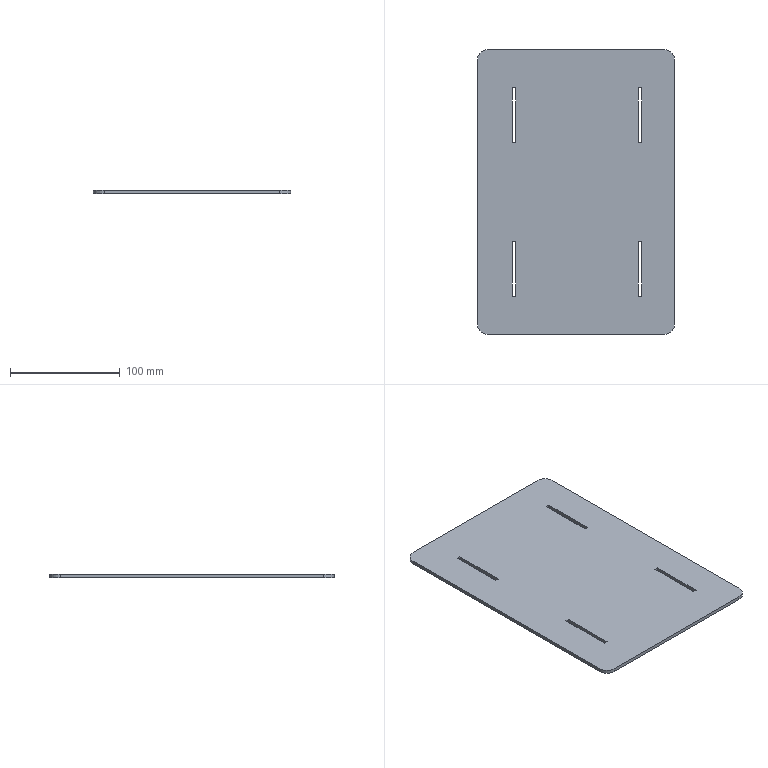Part | SolidWorks | features FlatPattern 1, SMBaseFlange 1, SheetMetal 1 | 1 solid | 26 faces | box 180 x 260 x 3.2 mm | volume 147437 mm3 | plane 22 | cylinder 4 | commonest cylinder face diameters 20 x4
STEP:
#1=CARTESIAN_POINT('',(-25.,119.865,3.2));
#2=VERTEX_POINT('',#1);
#3=CARTESIAN_POINT('',(-35.,109.865,3.2));
#4=VERTEX_POINT('',#3);
#5=CARTESIAN_POINT('',(-25.,109.865,3.2));
#6=DIRECTION('',(0.,0.,1.));
#7=DIRECTION('',(1.,0.,0.));
#8=AXIS2_PLACEMENT_3D('',#5,#6,#7);
#9=CIRCLE('',#8,10.);
#10=EDGE_CURVE('',#2,#4,#9,.T.);
#11=ORIENTED_EDGE('',*,*,#10,.T.);
#12=CARTESIAN_POINT('',(-35.,-130.135,3.2));
#13=VERTEX_POINT('',#12);
#14=CARTESIAN_POINT('',(-35.,109.865,3.2));
#15=DIRECTION('',(0.,-1.,0.));
#16=VECTOR('',#15,1000.);
#17=LINE('',#14,#16);
#18=EDGE_CURVE('',#4,#13,#17,.T.);
#19=ORIENTED_EDGE('',*,*,#18,.T.);
#20=CARTESIAN_POINT('',(-25.,-140.135,3.2));
#21=VERTEX_POINT('',#20);
#22=CARTESIAN_POINT('',(-25.,-130.135,3.2));
#23=DIRECTION('',(0.,0.,1.));
#24=DIRECTION('',(-1.,0.,0.));
#25=AXIS2_PLACEMENT_3D('',#22,#23,#24);
#26=CIRCLE('',#25,10.);
#27=EDGE_CURVE('',#13,#21,#26,.T.);
#28=ORIENTED_EDGE('',*,*,#27,.T.);
#29=CARTESIAN_POINT('',(135.,-140.135,3.2));
#30=VERTEX_POINT('',#29);
#31=CARTESIAN_POINT('',(135.,-140.135,3.2));
#32=DIRECTION('',(1.,0.,0.));
#33=VECTOR('',#32,1000.);
#34=LINE('',#31,#33);
#35=EDGE_CURVE('',#21,#30,#34,.T.);
#36=ORIENTED_EDGE('',*,*,#35,.T.);
#37=CARTESIAN_POINT('',(145.,-130.135,3.2));
#38=VERTEX_POINT('',#37);
#39=CARTESIAN_POINT('',(135.,-130.135,3.2));
#40=DIRECTION('',(0.,0.,1.));
#41=DIRECTION('',(-1.,0.,0.));
#42=AXIS2_PLACEMENT_3D('',#39,#40,#41);
#43=CIRCLE('',#42,10.);
#44=EDGE_CURVE('',#30,#38,#43,.T.);
#45=ORIENTED_EDGE('',*,*,#44,.T.);
#46=CARTESIAN_POINT('',(145.,109.865,3.2));
#47=VERTEX_POINT('',#46);
#48=CARTESIAN_POINT('',(145.,109.865,3.2));
#49=DIRECTION('',(0.,1.,0.));
#50=VECTOR('',#49,1000.);
#51=LINE('',#48,#50);
#52=EDGE_CURVE('',#38,#47,#51,.T.);
#53=ORIENTED_EDGE('',*,*,#52,.T.);
#54=CARTESIAN_POINT('',(135.,119.865,3.2));
#55=VERTEX_POINT('',#54);
#56=CARTESIAN_POINT('',(135.,109.865,3.2));
#57=DIRECTION('',(0.,0.,1.));
#58=DIRECTION('',(-1.,0.,0.));
#59=AXIS2_PLACEMENT_3D('',#56,#57,#58);
#60=CIRCLE('',#59,10.);
#61=EDGE_CURVE('',#47,#55,#60,.T.);
#62=ORIENTED_EDGE('',*,*,#61,.T.);
#63=CARTESIAN_POINT('',(135.,119.865,3.2));
#64=DIRECTION('',(-1.,0.,0.));
#65=VECTOR('',#64,1000.);
#66=LINE('',#63,#65);
#67=EDGE_CURVE('',#55,#2,#66,.T.);
#68=ORIENTED_EDGE('',*,*,#67,.T.);
#69=EDGE_LOOP('',(#11,#19,#28,#36,#45,#53,#62,#68));
#70=FACE_OUTER_BOUND('',#69,.T.);
#71=CARTESIAN_POINT('',(111.8,34.865,3.2));
#72=VERTEX_POINT('',#71);
#73=CARTESIAN_POINT('',(115.,34.865,3.2));
#74=VERTEX_POINT('',#73);
#75=CARTESIAN_POINT('',(111.8,34.865,3.2));
#76=DIRECTION('',(1.,0.,0.));
#77=VECTOR('',#76,1000.);
#78=LINE('',#75,#77);
#79=EDGE_CURVE('',#72,#74,#78,.T.);
#80=ORIENTED_EDGE('',*,*,#79,.F.);
#81=CARTESIAN_POINT('',(111.8,84.865,3.2));
#82=VERTEX_POINT('',#81);
#83=CARTESIAN_POINT('',(111.8,34.865,3.2));
#84=DIRECTION('',(0.,-1.,0.));
#85=VECTOR('',#84,1000.);
#86=LINE('',#83,#85);
#87=EDGE_CURVE('',#82,#72,#86,.T.);
#88=ORIENTED_EDGE('',*,*,#87,.F.);
#89=CARTESIAN_POINT('',(115.,84.865,3.2));
#90=VERTEX_POINT('',#89);
#91=CARTESIAN_POINT('',(111.8,84.865,3.2));
#92=DIRECTION('',(-1.,0.,0.));
#93=VECTOR('',#92,1000.);
#94=LINE('',#91,#93);
#95=EDGE_CURVE('',#90,#82,#94,.T.);
#96=ORIENTED_EDGE('',*,*,#95,.F.);
#97=CARTESIAN_POINT('',(115.,34.865,3.2));
#98=DIRECTION('',(0.,1.,0.));
#99=VECTOR('',#98,1000.);
#100=LINE('',#97,#99);
#101=EDGE_CURVE('',#74,#90,#100,.T.);
#102=ORIENTED_EDGE('',*,*,#101,.F.);
#103=EDGE_LOOP('',(#80,#88,#96,#102));
#104=FACE_BOUND('',#103,.T.);
#105=CARTESIAN_POINT('',(111.8,-105.135,3.2));
#106=VERTEX_POINT('',#105);
#107=CARTESIAN_POINT('',(115.,-105.135,3.2));
#108=VERTEX_POINT('',#107);
#109=CARTESIAN_POINT('',(111.8,-105.135,3.2));
#110=DIRECTION('',(1.,0.,0.));
#111=VECTOR('',#110,1000.);
#112=LINE('',#109,#111);
#113=EDGE_CURVE('',#106,#108,#112,.T.);
#114=ORIENTED_EDGE('',*,*,#113,.F.);
#115=CARTESIAN_POINT('',(111.8,-55.135,3.2));
#116=VERTEX_POINT('',#115);
#117=CARTESIAN_POINT('',(111.8,-55.135,3.2));
#118=DIRECTION('',(0.,-1.,0.));
#119=VECTOR('',#118,1000.);
#120=LINE('',#117,#119);
#121=EDGE_CURVE('',#116,#106,#120,.T.);
#122=ORIENTED_EDGE('',*,*,#121,.F.);
#123=CARTESIAN_POINT('',(115.,-55.135,3.2));
#124=VERTEX_POINT('',#123);
#125=CARTESIAN_POINT('',(111.8,-55.135,3.2));
#126=DIRECTION('',(-1.,0.,0.));
#127=VECTOR('',#126,1000.);
#128=LINE('',#125,#127);
#129=EDGE_CURVE('',#124,#116,#128,.T.);
#130=ORIENTED_EDGE('',*,*,#129,.F.);
#131=CARTESIAN_POINT('',(115.,-55.135,3.2));
#132=DIRECTION('',(0.,1.,0.));
#133=VECTOR('',#132,1000.);
#134=LINE('',#131,#133);
#135=EDGE_CURVE('',#108,#124,#134,.T.);
#136=ORIENTED_EDGE('',*,*,#135,.F.);
#137=EDGE_LOOP('',(#114,#122,#130,#136));
#138=FACE_BOUND('',#137,.T.);
#139=CARTESIAN_POINT('',(0.,-55.135,3.2));
#140=VERTEX_POINT('',#139);
#141=CARTESIAN_POINT('',(-3.2,-55.135,3.2));
#142=VERTEX_POINT('',#141);
#143=CARTESIAN_POINT('',(0.,-55.135,3.2));
#144=DIRECTION('',(-1.,0.,0.));
#145=VECTOR('',#144,1000.);
#146=LINE('',#143,#145);
#147=EDGE_CURVE('',#140,#142,#146,.T.);
#148=ORIENTED_EDGE('',*,*,#147,.F.);
#149=CARTESIAN_POINT('',(0.,-105.135,3.2));
#150=VERTEX_POINT('',#149);
#151=CARTESIAN_POINT('',(0.,-55.135,3.2));
#152=DIRECTION('',(0.,1.,0.));
#153=VECTOR('',#152,1000.);
#154=LINE('',#151,#153);
#155=EDGE_CURVE('',#150,#140,#154,.T.);
#156=ORIENTED_EDGE('',*,*,#155,.F.);
#157=CARTESIAN_POINT('',(-3.2,-105.135,3.2));
#158=VERTEX_POINT('',#157);
#159=CARTESIAN_POINT('',(0.,-105.135,3.2));
#160=DIRECTION('',(1.,0.,0.));
#161=VECTOR('',#160,1000.);
#162=LINE('',#159,#161);
#163=EDGE_CURVE('',#158,#150,#162,.T.);
#164=ORIENTED_EDGE('',*,*,#163,.F.);
#165=CARTESIAN_POINT('',(-3.2,-55.135,3.2));
#166=DIRECTION('',(0.,-1.,0.));
#167=VECTOR('',#166,1000.);
#168=LINE('',#165,#167);
#169=EDGE_CURVE('',#142,#158,#168,.T.);
#170=ORIENTED_EDGE('',*,*,#169,.F.);
#171=EDGE_LOOP('',(#148,#156,#164,#170));
#172=FACE_BOUND('',#171,.T.);
#173=CARTESIAN_POINT('',(0.,84.865,3.2));
#174=VERTEX_POINT('',#173);
#175=CARTESIAN_POINT('',(-3.2,84.865,3.2));
#176=VERTEX_POINT('',#175);
#177=CARTESIAN_POINT('',(0.,84.865,3.2));
#178=DIRECTION('',(-1.,0.,0.));
#179=VECTOR('',#178,1000.);
#180=LINE('',#177,#179);
#181=EDGE_CURVE('',#174,#176,#180,.T.);
#182=ORIENTED_EDGE('',*,*,#181,.F.);
#183=CARTESIAN_POINT('',(0.,34.865,3.2));
#184=VERTEX_POINT('',#183);
#185=CARTESIAN_POINT('',(0.,34.865,3.2));
#186=DIRECTION('',(0.,1.,0.));
#187=VECTOR('',#186,1000.);
#188=LINE('',#185,#187);
#189=EDGE_CURVE('',#184,#174,#188,.T.);
#190=ORIENTED_EDGE('',*,*,#189,.F.);
#191=CARTESIAN_POINT('',(-3.2,34.865,3.2));
#192=VERTEX_POINT('',#191);
#193=CARTESIAN_POINT('',(0.,34.865,3.2));
#194=DIRECTION('',(1.,0.,0.));
#195=VECTOR('',#194,1000.);
#196=LINE('',#193,#195);
#197=EDGE_CURVE('',#192,#184,#196,.T.);
#198=ORIENTED_EDGE('',*,*,#197,.F.);
#199=CARTESIAN_POINT('',(-3.2,34.865,3.2));
#200=DIRECTION('',(0.,-1.,0.));
#201=VECTOR('',#200,1000.);
#202=LINE('',#199,#201);
#203=EDGE_CURVE('',#176,#192,#202,.T.);
#204=ORIENTED_EDGE('',*,*,#203,.F.);
#205=EDGE_LOOP('',(#182,#190,#198,#204));
#206=FACE_BOUND('',#205,.T.);
#207=CARTESIAN_POINT('',(-25.,109.865,3.2));
#208=DIRECTION('',(0.,0.,1.));
#209=DIRECTION('',(1.,0.,0.));
#210=AXIS2_PLACEMENT_3D('',#207,#208,#209);
#211=PLANE('',#210);
#212=ADVANCED_FACE('',(#70,#104,#138,#172,#206),#211,.T.);
#213=CARTESIAN_POINT('',(0.,-105.135,0.));
#214=VERTEX_POINT('',#213);
#215=CARTESIAN_POINT('',(0.,-55.135,0.));
#216=VERTEX_POINT('',#215);
#217=CARTESIAN_POINT('',(0.,-55.135,0.));
#218=DIRECTION('',(0.,1.,0.));
#219=VECTOR('',#218,1000.);
#220=LINE('',#217,#219);
#221=EDGE_CURVE('',#214,#216,#220,.T.);
#222=ORIENTED_EDGE('',*,*,#221,.T.);
#223=CARTESIAN_POINT('',(-3.2,-55.135,0.));
#224=VERTEX_POINT('',#223);
#225=CARTESIAN_POINT('',(0.,-55.135,0.));
#226=DIRECTION('',(-1.,0.,0.));
#227=VECTOR('',#226,1000.);
#228=LINE('',#225,#227);
#229=EDGE_CURVE('',#216,#224,#228,.T.);
#230=ORIENTED_EDGE('',*,*,#229,.T.);
#231=CARTESIAN_POINT('',(-3.2,-105.135,0.));
#232=VERTEX_POINT('',#231);
#233=CARTESIAN_POINT('',(-3.2,-55.135,0.));
#234=DIRECTION('',(0.,-1.,0.));
#235=VECTOR('',#234,1000.);
#236=LINE('',#233,#235);
#237=EDGE_CURVE('',#224,#232,#236,.T.);
#238=ORIENTED_EDGE('',*,*,#237,.T.);
#239=CARTESIAN_POINT('',(0.,-105.135,0.));
#240=DIRECTION('',(1.,0.,0.));
#241=VECTOR('',#240,1000.);
#242=LINE('',#239,#241);
#243=EDGE_CURVE('',#232,#214,#242,.T.);
#244=ORIENTED_EDGE('',*,*,#243,.T.);
#245=EDGE_LOOP('',(#222,#230,#238,#244));
#246=FACE_BOUND('',#245,.T.);
#247=CARTESIAN_POINT('',(111.8,84.865,0.));
#248=VERTEX_POINT('',#247);
#249=CARTESIAN_POINT('',(111.8,34.865,0.));
#250=VERTEX_POINT('',#249);
#251=CARTESIAN_POINT('',(111.8,34.865,0.));
#252=DIRECTION('',(0.,-1.,0.));
#253=VECTOR('',#252,1000.);
#254=LINE('',#251,#253);
#255=EDGE_CURVE('',#248,#250,#254,.T.);
#256=ORIENTED_EDGE('',*,*,#255,.T.);
#257=CARTESIAN_POINT('',(115.,34.865,0.));
#258=VERTEX_POINT('',#257);
#259=CARTESIAN_POINT('',(111.8,34.865,0.));
#260=DIRECTION('',(1.,0.,0.));
#261=VECTOR('',#260,1000.);
#262=LINE('',#259,#261);
#263=EDGE_CURVE('',#250,#258,#262,.T.);
#264=ORIENTED_EDGE('',*,*,#263,.T.);
#265=CARTESIAN_POINT('',(115.,84.865,0.));
#266=VERTEX_POINT('',#265);
#267=CARTESIAN_POINT('',(115.,34.865,0.));
#268=DIRECTION('',(0.,1.,0.));
#269=VECTOR('',#268,1000.);
#270=LINE('',#267,#269);
#271=EDGE_CURVE('',#258,#266,#270,.T.);
#272=ORIENTED_EDGE('',*,*,#271,.T.);
#273=CARTESIAN_POINT('',(111.8,84.865,0.));
#274=DIRECTION('',(-1.,0.,0.));
#275=VECTOR('',#274,1000.);
#276=LINE('',#273,#275);
#277=EDGE_CURVE('',#266,#248,#276,.T.);
#278=ORIENTED_EDGE('',*,*,#277,.T.);
#279=EDGE_LOOP('',(#256,#264,#272,#278));
#280=FACE_BOUND('',#279,.T.);
#281=CARTESIAN_POINT('',(-25.,119.865,0.));
#282=VERTEX_POINT('',#281);
#283=CARTESIAN_POINT('',(-35.,109.865,0.));
#284=VERTEX_POINT('',#283);
#285=CARTESIAN_POINT('',(-25.,109.865,0.));
#286=DIRECTION('',(0.,0.,1.));
#287=DIRECTION('',(1.,0.,0.));
#288=AXIS2_PLACEMENT_3D('',#285,#286,#287);
#289=CIRCLE('',#288,10.);
#290=EDGE_CURVE('',#282,#284,#289,.T.);
#291=ORIENTED_EDGE('',*,*,#290,.F.);
#292=CARTESIAN_POINT('',(135.,119.865,0.));
#293=VERTEX_POINT('',#292);
#294=CARTESIAN_POINT('',(135.,119.865,0.));
#295=DIRECTION('',(-1.,0.,0.));
#296=VECTOR('',#295,1000.);
#297=LINE('',#294,#296);
#298=EDGE_CURVE('',#293,#282,#297,.T.);
#299=ORIENTED_EDGE('',*,*,#298,.F.);
#300=CARTESIAN_POINT('',(145.,109.865,0.));
#301=VERTEX_POINT('',#300);
#302=CARTESIAN_POINT('',(135.,109.865,0.));
#303=DIRECTION('',(0.,0.,1.));
#304=DIRECTION('',(-1.,0.,0.));
#305=AXIS2_PLACEMENT_3D('',#302,#303,#304);
#306=CIRCLE('',#305,10.);
#307=EDGE_CURVE('',#301,#293,#306,.T.);
#308=ORIENTED_EDGE('',*,*,#307,.F.);
#309=CARTESIAN_POINT('',(145.,-130.135,0.));
#310=VERTEX_POINT('',#309);
#311=CARTESIAN_POINT('',(145.,109.865,0.));
#312=DIRECTION('',(0.,1.,0.));
#313=VECTOR('',#312,1000.);
#314=LINE('',#311,#313);
#315=EDGE_CURVE('',#310,#301,#314,.T.);
#316=ORIENTED_EDGE('',*,*,#315,.F.);
#317=CARTESIAN_POINT('',(135.,-140.135,0.));
#318=VERTEX_POINT('',#317);
#319=CARTESIAN_POINT('',(135.,-130.135,0.));
#320=DIRECTION('',(0.,0.,1.));
#321=DIRECTION('',(-1.,0.,0.));
#322=AXIS2_PLACEMENT_3D('',#319,#320,#321);
#323=CIRCLE('',#322,10.);
#324=EDGE_CURVE('',#318,#310,#323,.T.);
#325=ORIENTED_EDGE('',*,*,#324,.F.);
#326=CARTESIAN_POINT('',(-25.,-140.135,0.));
#327=VERTEX_POINT('',#326);
#328=CARTESIAN_POINT('',(135.,-140.135,0.));
#329=DIRECTION('',(1.,0.,0.));
#330=VECTOR('',#329,1000.);
#331=LINE('',#328,#330);
#332=EDGE_CURVE('',#327,#318,#331,.T.);
#333=ORIENTED_EDGE('',*,*,#332,.F.);
#334=CARTESIAN_POINT('',(-35.,-130.135,0.));
#335=VERTEX_POINT('',#334);
#336=CARTESIAN_POINT('',(-25.,-130.135,0.));
#337=DIRECTION('',(0.,0.,1.));
#338=DIRECTION('',(-1.,0.,0.));
#339=AXIS2_PLACEMENT_3D('',#336,#337,#338);
#340=CIRCLE('',#339,10.);
#341=EDGE_CURVE('',#335,#327,#340,.T.);
#342=ORIENTED_EDGE('',*,*,#341,.F.);
#343=CARTESIAN_POINT('',(-35.,109.865,0.));
#344=DIRECTION('',(0.,-1.,0.));
#345=VECTOR('',#344,1000.);
#346=LINE('',#343,#345);
#347=EDGE_CURVE('',#284,#335,#346,.T.);
#348=ORIENTED_EDGE('',*,*,#347,.F.);
#349=EDGE_LOOP('',(#291,#299,#308,#316,#325,#333,#342,#348));
#350=FACE_OUTER_BOUND('',#349,.T.);
#351=CARTESIAN_POINT('',(111.8,-55.135,0.));
#352=VERTEX_POINT('',#351);
#353=CARTESIAN_POINT('',(111.8,-105.135,0.));
#354=VERTEX_POINT('',#353);
#355=CARTESIAN_POINT('',(111.8,-55.135,0.));
#356=DIRECTION('',(0.,-1.,0.));
#357=VECTOR('',#356,1000.);
#358=LINE('',#355,#357);
#359=EDGE_CURVE('',#352,#354,#358,.T.);
#360=ORIENTED_EDGE('',*,*,#359,.T.);
#361=CARTESIAN_POINT('',(115.,-105.135,0.));
#362=VERTEX_POINT('',#361);
#363=CARTESIAN_POINT('',(111.8,-105.135,0.));
#364=DIRECTION('',(1.,0.,0.));
#365=VECTOR('',#364,1000.);
#366=LINE('',#363,#365);
#367=EDGE_CURVE('',#354,#362,#366,.T.);
#368=ORIENTED_EDGE('',*,*,#367,.T.);
#369=CARTESIAN_POINT('',(115.,-55.135,0.));
#370=VERTEX_POINT('',#369);
#371=CARTESIAN_POINT('',(115.,-55.135,0.));
#372=DIRECTION('',(0.,1.,0.));
#373=VECTOR('',#372,1000.);
#374=LINE('',#371,#373);
#375=EDGE_CURVE('',#362,#370,#374,.T.);
#376=ORIENTED_EDGE('',*,*,#375,.T.);
#377=CARTESIAN_POINT('',(111.8,-55.135,0.));
#378=DIRECTION('',(-1.,0.,0.));
#379=VECTOR('',#378,1000.);
#380=LINE('',#377,#379);
#381=EDGE_CURVE('',#370,#352,#380,.T.);
#382=ORIENTED_EDGE('',*,*,#381,.T.);
#383=EDGE_LOOP('',(#360,#368,#376,#382));
#384=FACE_BOUND('',#383,.T.);
#385=CARTESIAN_POINT('',(0.,34.865,0.));
#386=VERTEX_POINT('',#385);
#387=CARTESIAN_POINT('',(0.,84.865,0.));
#388=VERTEX_POINT('',#387);
#389=CARTESIAN_POINT('',(0.,34.865,0.));
#390=DIRECTION('',(0.,1.,0.));
#391=VECTOR('',#390,1000.);
#392=LINE('',#389,#391);
#393=EDGE_CURVE('',#386,#388,#392,.T.);
#394=ORIENTED_EDGE('',*,*,#393,.T.);
#395=CARTESIAN_POINT('',(-3.2,84.865,0.));
#396=VERTEX_POINT('',#395);
#397=CARTESIAN_POINT('',(0.,84.865,0.));
#398=DIRECTION('',(-1.,0.,0.));
#399=VECTOR('',#398,1000.);
#400=LINE('',#397,#399);
#401=EDGE_CURVE('',#388,#396,#400,.T.);
#402=ORIENTED_EDGE('',*,*,#401,.T.);
#403=CARTESIAN_POINT('',(-3.2,34.865,0.));
#404=VERTEX_POINT('',#403);
#405=CARTESIAN_POINT('',(-3.2,34.865,0.));
#406=DIRECTION('',(0.,-1.,0.));
#407=VECTOR('',#406,1000.);
#408=LINE('',#405,#407);
#409=EDGE_CURVE('',#396,#404,#408,.T.);
#410=ORIENTED_EDGE('',*,*,#409,.T.);
#411=CARTESIAN_POINT('',(0.,34.865,0.));
#412=DIRECTION('',(1.,0.,0.));
#413=VECTOR('',#412,1000.);
#414=LINE('',#411,#413);
#415=EDGE_CURVE('',#404,#386,#414,.T.);
#416=ORIENTED_EDGE('',*,*,#415,.T.);
#417=EDGE_LOOP('',(#394,#402,#410,#416));
#418=FACE_BOUND('',#417,.T.);
#419=CARTESIAN_POINT('',(-25.,109.865,0.));
#420=DIRECTION('',(0.,0.,1.));
#421=DIRECTION('',(1.,0.,0.));
#422=AXIS2_PLACEMENT_3D('',#419,#420,#421);
#423=PLANE('',#422);
#424=ADVANCED_FACE('',(#246,#280,#350,#384,#418),#423,.F.);
#425=ORIENTED_EDGE('',*,*,#290,.T.);
#426=CARTESIAN_POINT('',(-35.,109.865,3.2));
#427=DIRECTION('',(0.,0.,-1.));
#428=VECTOR('',#427,1000.);
#429=LINE('',#426,#428);
#430=EDGE_CURVE('',#4,#284,#429,.T.);
#431=ORIENTED_EDGE('',*,*,#430,.F.);
#432=ORIENTED_EDGE('',*,*,#10,.F.);
#433=CARTESIAN_POINT('',(-25.,119.865,3.2));
#434=DIRECTION('',(0.,0.,-1.));
#435=VECTOR('',#434,1000.);
#436=LINE('',#433,#435);
#437=EDGE_CURVE('',#2,#282,#436,.T.);
#438=ORIENTED_EDGE('',*,*,#437,.T.);
#439=EDGE_LOOP('',(#425,#431,#432,#438));
#440=FACE_OUTER_BOUND('',#439,.T.);
#441=CARTESIAN_POINT('',(-25.,109.865,3.2));
#442=DIRECTION('',(0.,0.,-1.));
#443=DIRECTION('',(-1.,0.,0.));
#444=AXIS2_PLACEMENT_3D('',#441,#442,#443);
#445=CYLINDRICAL_SURFACE('',#444,10.);
#446=ADVANCED_FACE('',(#440),#445,.T.);
#447=ORIENTED_EDGE('',*,*,#347,.T.);
#448=CARTESIAN_POINT('',(-35.,-130.135,3.2));
#449=DIRECTION('',(0.,0.,-1.));
#450=VECTOR('',#449,1000.);
#451=LINE('',#448,#450);
#452=EDGE_CURVE('',#13,#335,#451,.T.);
#453=ORIENTED_EDGE('',*,*,#452,.F.);
#454=ORIENTED_EDGE('',*,*,#18,.F.);
#455=ORIENTED_EDGE('',*,*,#430,.T.);
#456=EDGE_LOOP('',(#447,#453,#454,#455));
#457=FACE_OUTER_BOUND('',#456,.T.);
#458=CARTESIAN_POINT('',(-35.,109.865,3.2));
#459=DIRECTION('',(1.,0.,0.));
#460=DIRECTION('',(0.,1.,0.));
#461=AXIS2_PLACEMENT_3D('',#458,#459,#460);
#462=PLANE('',#461);
#463=ADVANCED_FACE('',(#457),#462,.F.);
#464=ORIENTED_EDGE('',*,*,#341,.T.);
#465=CARTESIAN_POINT('',(-25.,-140.135,3.2));
#466=DIRECTION('',(0.,0.,-1.));
#467=VECTOR('',#466,1000.);
#468=LINE('',#465,#467);
#469=EDGE_CURVE('',#21,#327,#468,.T.);
#470=ORIENTED_EDGE('',*,*,#469,.F.);
#471=ORIENTED_EDGE('',*,*,#27,.F.);
#472=ORIENTED_EDGE('',*,*,#452,.T.);
#473=EDGE_LOOP('',(#464,#470,#471,#472));
#474=FACE_OUTER_BOUND('',#473,.T.);
#475=CARTESIAN_POINT('',(-25.,-130.135,3.2));
#476=DIRECTION('',(0.,0.,-1.));
#477=DIRECTION('',(-1.,0.,0.));
#478=AXIS2_PLACEMENT_3D('',#475,#476,#477);
#479=CYLINDRICAL_SURFACE('',#478,10.);
#480=ADVANCED_FACE('',(#474),#479,.T.);
#481=ORIENTED_EDGE('',*,*,#332,.T.);
#482=CARTESIAN_POINT('',(135.,-140.135,3.2));
#483=DIRECTION('',(0.,0.,-1.));
#484=VECTOR('',#483,1000.);
#485=LINE('',#482,#484);
#486=EDGE_CURVE('',#30,#318,#485,.T.);
#487=ORIENTED_EDGE('',*,*,#486,.F.);
#488=ORIENTED_EDGE('',*,*,#35,.F.);
#489=ORIENTED_EDGE('',*,*,#469,.T.);
#490=EDGE_LOOP('',(#481,#487,#488,#489));
#491=FACE_OUTER_BOUND('',#490,.T.);
#492=CARTESIAN_POINT('',(135.,-140.135,3.2));
#493=DIRECTION('',(0.,1.,0.));
#494=DIRECTION('',(0.,0.,1.));
#495=AXIS2_PLACEMENT_3D('',#492,#493,#494);
#496=PLANE('',#495);
#497=ADVANCED_FACE('',(#491),#496,.F.);
#498=ORIENTED_EDGE('',*,*,#324,.T.);
#499=CARTESIAN_POINT('',(145.,-130.135,3.2));
#500=DIRECTION('',(0.,0.,-1.));
#501=VECTOR('',#500,1000.);
#502=LINE('',#499,#501);
#503=EDGE_CURVE('',#38,#310,#502,.T.);
#504=ORIENTED_EDGE('',*,*,#503,.F.);
#505=ORIENTED_EDGE('',*,*,#44,.F.);
#506=ORIENTED_EDGE('',*,*,#486,.T.);
#507=EDGE_LOOP('',(#498,#504,#505,#506));
#508=FACE_OUTER_BOUND('',#507,.T.);
#509=CARTESIAN_POINT('',(135.,-130.135,3.2));
#510=DIRECTION('',(0.,0.,-1.));
#511=DIRECTION('',(-1.,0.,0.));
#512=AXIS2_PLACEMENT_3D('',#509,#510,#511);
#513=CYLINDRICAL_SURFACE('',#512,10.);
#514=ADVANCED_FACE('',(#508),#513,.T.);
#515=ORIENTED_EDGE('',*,*,#315,.T.);
#516=CARTESIAN_POINT('',(145.,109.865,3.2));
#517=DIRECTION('',(0.,0.,-1.));
#518=VECTOR('',#517,1000.);
#519=LINE('',#516,#518);
#520=EDGE_CURVE('',#47,#301,#519,.T.);
#521=ORIENTED_EDGE('',*,*,#520,.F.);
#522=ORIENTED_EDGE('',*,*,#52,.F.);
#523=ORIENTED_EDGE('',*,*,#503,.T.);
#524=EDGE_LOOP('',(#515,#521,#522,#523));
#525=FACE_OUTER_BOUND('',#524,.T.);
#526=CARTESIAN_POINT('',(145.,109.865,3.2));
#527=DIRECTION('',(-1.,0.,0.));
#528=DIRECTION('',(0.,-1.,0.));
#529=AXIS2_PLACEMENT_3D('',#526,#527,#528);
#530=PLANE('',#529);
#531=ADVANCED_FACE('',(#525),#530,.F.);
#532=ORIENTED_EDGE('',*,*,#307,.T.);
#533=CARTESIAN_POINT('',(135.,119.865,3.2));
#534=DIRECTION('',(0.,0.,-1.));
#535=VECTOR('',#534,1000.);
#536=LINE('',#533,#535);
#537=EDGE_CURVE('',#55,#293,#536,.T.);
#538=ORIENTED_EDGE('',*,*,#537,.F.);
#539=ORIENTED_EDGE('',*,*,#61,.F.);
#540=ORIENTED_EDGE('',*,*,#520,.T.);
#541=EDGE_LOOP('',(#532,#538,#539,#540));
#542=FACE_OUTER_BOUND('',#541,.T.);
#543=CARTESIAN_POINT('',(135.,109.865,3.2));
#544=DIRECTION('',(0.,0.,-1.));
#545=DIRECTION('',(-1.,0.,0.));
#546=AXIS2_PLACEMENT_3D('',#543,#544,#545);
#547=CYLINDRICAL_SURFACE('',#546,10.);
#548=ADVANCED_FACE('',(#542),#547,.T.);
#549=ORIENTED_EDGE('',*,*,#298,.T.);
#550=ORIENTED_EDGE('',*,*,#437,.F.);
#551=ORIENTED_EDGE('',*,*,#67,.F.);
#552=ORIENTED_EDGE('',*,*,#537,.T.);
#553=EDGE_LOOP('',(#549,#550,#551,#552));
#554=FACE_OUTER_BOUND('',#553,.T.);
#555=CARTESIAN_POINT('',(135.,119.865,3.2));
#556=DIRECTION('',(0.,-1.,0.));
#557=DIRECTION('',(1.,0.,0.));
#558=AXIS2_PLACEMENT_3D('',#555,#556,#557);
#559=PLANE('',#558);
#560=ADVANCED_FACE('',(#554),#559,.F.);
#561=ORIENTED_EDGE('',*,*,#255,.F.);
#562=CARTESIAN_POINT('',(111.8,84.865,3.2));
#563=DIRECTION('',(0.,0.,-1.));
#564=VECTOR('',#563,1000.);
#565=LINE('',#562,#564);
#566=EDGE_CURVE('',#82,#248,#565,.T.);
#567=ORIENTED_EDGE('',*,*,#566,.F.);
#568=ORIENTED_EDGE('',*,*,#87,.T.);
#569=CARTESIAN_POINT('',(111.8,34.865,3.2));
#570=DIRECTION('',(0.,0.,-1.));
#571=VECTOR('',#570,1000.);
#572=LINE('',#569,#571);
#573=EDGE_CURVE('',#72,#250,#572,.T.);
#574=ORIENTED_EDGE('',*,*,#573,.T.);
#575=EDGE_LOOP('',(#561,#567,#568,#574));
#576=FACE_OUTER_BOUND('',#575,.T.);
#577=CARTESIAN_POINT('',(111.8,34.865,3.2));
#578=DIRECTION('',(1.,0.,0.));
#579=DIRECTION('',(0.,0.,-1.));
#580=AXIS2_PLACEMENT_3D('',#577,#578,#579);
#581=PLANE('',#580);
#582=ADVANCED_FACE('',(#576),#581,.T.);
#583=ORIENTED_EDGE('',*,*,#263,.F.);
#584=ORIENTED_EDGE('',*,*,#573,.F.);
#585=ORIENTED_EDGE('',*,*,#79,.T.);
#586=CARTESIAN_POINT('',(115.,34.865,3.2));
#587=DIRECTION('',(0.,0.,-1.));
#588=VECTOR('',#587,1000.);
#589=LINE('',#586,#588);
#590=EDGE_CURVE('',#74,#258,#589,.T.);
#591=ORIENTED_EDGE('',*,*,#590,.T.);
#592=EDGE_LOOP('',(#583,#584,#585,#591));
#593=FACE_OUTER_BOUND('',#592,.T.);
#594=CARTESIAN_POINT('',(111.8,34.865,3.2));
#595=DIRECTION('',(0.,1.,0.));
#596=DIRECTION('',(0.,0.,1.));
#597=AXIS2_PLACEMENT_3D('',#594,#595,#596);
#598=PLANE('',#597);
#599=ADVANCED_FACE('',(#593),#598,.T.);
#600=ORIENTED_EDGE('',*,*,#271,.F.);
#601=ORIENTED_EDGE('',*,*,#590,.F.);
#602=ORIENTED_EDGE('',*,*,#101,.T.);
#603=CARTESIAN_POINT('',(115.,84.865,3.2));
#604=DIRECTION('',(0.,0.,-1.));
#605=VECTOR('',#604,1000.);
#606=LINE('',#603,#605);
#607=EDGE_CURVE('',#90,#266,#606,.T.);
#608=ORIENTED_EDGE('',*,*,#607,.T.);
#609=EDGE_LOOP('',(#600,#601,#602,#608));
#610=FACE_OUTER_BOUND('',#609,.T.);
#611=CARTESIAN_POINT('',(115.,34.865,3.2));
#612=DIRECTION('',(-1.,0.,0.));
#613=DIRECTION('',(0.,0.,1.));
#614=AXIS2_PLACEMENT_3D('',#611,#612,#613);
#615=PLANE('',#614);
#616=ADVANCED_FACE('',(#610),#615,.T.);
#617=ORIENTED_EDGE('',*,*,#277,.F.);
#618=ORIENTED_EDGE('',*,*,#607,.F.);
#619=ORIENTED_EDGE('',*,*,#95,.T.);
#620=ORIENTED_EDGE('',*,*,#566,.T.);
#621=EDGE_LOOP('',(#617,#618,#619,#620));
#622=FACE_OUTER_BOUND('',#621,.T.);
#623=CARTESIAN_POINT('',(111.8,84.865,3.2));
#624=DIRECTION('',(0.,-1.,0.));
#625=DIRECTION('',(0.,0.,-1.));
#626=AXIS2_PLACEMENT_3D('',#623,#624,#625);
#627=PLANE('',#626);
#628=ADVANCED_FACE('',(#622),#627,.T.);
#629=ORIENTED_EDGE('',*,*,#359,.F.);
#630=CARTESIAN_POINT('',(111.8,-55.135,3.2));
#631=DIRECTION('',(0.,0.,-1.));
#632=VECTOR('',#631,1000.);
#633=LINE('',#630,#632);
#634=EDGE_CURVE('',#116,#352,#633,.T.);
#635=ORIENTED_EDGE('',*,*,#634,.F.);
#636=ORIENTED_EDGE('',*,*,#121,.T.);
#637=CARTESIAN_POINT('',(111.8,-105.135,3.2));
#638=DIRECTION('',(0.,0.,-1.));
#639=VECTOR('',#638,1000.);
#640=LINE('',#637,#639);
#641=EDGE_CURVE('',#106,#354,#640,.T.);
#642=ORIENTED_EDGE('',*,*,#641,.T.);
#643=EDGE_LOOP('',(#629,#635,#636,#642));
#644=FACE_OUTER_BOUND('',#643,.T.);
#645=CARTESIAN_POINT('',(111.8,-55.135,3.2));
#646=DIRECTION('',(1.,0.,0.));
#647=DIRECTION('',(0.,0.,-1.));
#648=AXIS2_PLACEMENT_3D('',#645,#646,#647);
#649=PLANE('',#648);
#650=ADVANCED_FACE('',(#644),#649,.T.);
#651=ORIENTED_EDGE('',*,*,#367,.F.);
#652=ORIENTED_EDGE('',*,*,#641,.F.);
#653=ORIENTED_EDGE('',*,*,#113,.T.);
#654=CARTESIAN_POINT('',(115.,-105.135,3.2));
#655=DIRECTION('',(0.,0.,-1.));
#656=VECTOR('',#655,1000.);
#657=LINE('',#654,#656);
#658=EDGE_CURVE('',#108,#362,#657,.T.);
#659=ORIENTED_EDGE('',*,*,#658,.T.);
#660=EDGE_LOOP('',(#651,#652,#653,#659));
#661=FACE_OUTER_BOUND('',#660,.T.);
#662=CARTESIAN_POINT('',(111.8,-105.135,3.2));
#663=DIRECTION('',(0.,1.,0.));
#664=DIRECTION('',(0.,0.,1.));
#665=AXIS2_PLACEMENT_3D('',#662,#663,#664);
#666=PLANE('',#665);
#667=ADVANCED_FACE('',(#661),#666,.T.);
#668=ORIENTED_EDGE('',*,*,#375,.F.);
#669=ORIENTED_EDGE('',*,*,#658,.F.);
#670=ORIENTED_EDGE('',*,*,#135,.T.);
#671=CARTESIAN_POINT('',(115.,-55.135,3.2));
#672=DIRECTION('',(0.,0.,-1.));
#673=VECTOR('',#672,1000.);
#674=LINE('',#671,#673);
#675=EDGE_CURVE('',#124,#370,#674,.T.);
#676=ORIENTED_EDGE('',*,*,#675,.T.);
#677=EDGE_LOOP('',(#668,#669,#670,#676));
#678=FACE_OUTER_BOUND('',#677,.T.);
#679=CARTESIAN_POINT('',(115.,-55.135,3.2));
#680=DIRECTION('',(-1.,0.,0.));
#681=DIRECTION('',(0.,0.,1.));
#682=AXIS2_PLACEMENT_3D('',#679,#680,#681);
#683=PLANE('',#682);
#684=ADVANCED_FACE('',(#678),#683,.T.);
#685=ORIENTED_EDGE('',*,*,#381,.F.);
#686=ORIENTED_EDGE('',*,*,#675,.F.);
#687=ORIENTED_EDGE('',*,*,#129,.T.);
#688=ORIENTED_EDGE('',*,*,#634,.T.);
#689=EDGE_LOOP('',(#685,#686,#687,#688));
#690=FACE_OUTER_BOUND('',#689,.T.);
#691=CARTESIAN_POINT('',(111.8,-55.135,3.2));
#692=DIRECTION('',(0.,-1.,0.));
#693=DIRECTION('',(0.,0.,-1.));
#694=AXIS2_PLACEMENT_3D('',#691,#692,#693);
#695=PLANE('',#694);
#696=ADVANCED_FACE('',(#690),#695,.T.);
#697=ORIENTED_EDGE('',*,*,#221,.F.);
#698=CARTESIAN_POINT('',(0.,-105.135,3.2));
#699=DIRECTION('',(0.,0.,-1.));
#700=VECTOR('',#699,1000.);
#701=LINE('',#698,#700);
#702=EDGE_CURVE('',#150,#214,#701,.T.);
#703=ORIENTED_EDGE('',*,*,#702,.F.);
#704=ORIENTED_EDGE('',*,*,#155,.T.);
#705=CARTESIAN_POINT('',(0.,-55.135,3.2));
#706=DIRECTION('',(0.,0.,-1.));
#707=VECTOR('',#706,1000.);
#708=LINE('',#705,#707);
#709=EDGE_CURVE('',#140,#216,#708,.T.);
#710=ORIENTED_EDGE('',*,*,#709,.T.);
#711=EDGE_LOOP('',(#697,#703,#704,#710));
#712=FACE_OUTER_BOUND('',#711,.T.);
#713=CARTESIAN_POINT('',(0.,-55.135,3.2));
#714=DIRECTION('',(-1.,0.,0.));
#715=DIRECTION('',(0.,0.,1.));
#716=AXIS2_PLACEMENT_3D('',#713,#714,#715);
#717=PLANE('',#716);
#718=ADVANCED_FACE('',(#712),#717,.T.);
#719=ORIENTED_EDGE('',*,*,#229,.F.);
#720=ORIENTED_EDGE('',*,*,#709,.F.);
#721=ORIENTED_EDGE('',*,*,#147,.T.);
#722=CARTESIAN_POINT('',(-3.2,-55.135,3.2));
#723=DIRECTION('',(0.,0.,-1.));
#724=VECTOR('',#723,1000.);
#725=LINE('',#722,#724);
#726=EDGE_CURVE('',#142,#224,#725,.T.);
#727=ORIENTED_EDGE('',*,*,#726,.T.);
#728=EDGE_LOOP('',(#719,#720,#721,#727));
#729=FACE_OUTER_BOUND('',#728,.T.);
#730=CARTESIAN_POINT('',(0.,-55.135,3.2));
#731=DIRECTION('',(0.,-1.,0.));
#732=DIRECTION('',(0.,0.,-1.));
#733=AXIS2_PLACEMENT_3D('',#730,#731,#732);
#734=PLANE('',#733);
#735=ADVANCED_FACE('',(#729),#734,.T.);
#736=ORIENTED_EDGE('',*,*,#237,.F.);
#737=ORIENTED_EDGE('',*,*,#726,.F.);
#738=ORIENTED_EDGE('',*,*,#169,.T.);
#739=CARTESIAN_POINT('',(-3.2,-105.135,3.2));
#740=DIRECTION('',(0.,0.,-1.));
#741=VECTOR('',#740,1000.);
#742=LINE('',#739,#741);
#743=EDGE_CURVE('',#158,#232,#742,.T.);
#744=ORIENTED_EDGE('',*,*,#743,.T.);
#745=EDGE_LOOP('',(#736,#737,#738,#744));
#746=FACE_OUTER_BOUND('',#745,.T.);
#747=CARTESIAN_POINT('',(-3.2,-55.135,3.2));
#748=DIRECTION('',(1.,0.,0.));
#749=DIRECTION('',(0.,0.,-1.));
#750=AXIS2_PLACEMENT_3D('',#747,#748,#749);
#751=PLANE('',#750);
#752=ADVANCED_FACE('',(#746),#751,.T.);
#753=ORIENTED_EDGE('',*,*,#243,.F.);
#754=ORIENTED_EDGE('',*,*,#743,.F.);
#755=ORIENTED_EDGE('',*,*,#163,.T.);
#756=ORIENTED_EDGE('',*,*,#702,.T.);
#757=EDGE_LOOP('',(#753,#754,#755,#756));
#758=FACE_OUTER_BOUND('',#757,.T.);
#759=CARTESIAN_POINT('',(0.,-105.135,3.2));
#760=DIRECTION('',(0.,1.,0.));
#761=DIRECTION('',(0.,0.,1.));
#762=AXIS2_PLACEMENT_3D('',#759,#760,#761);
#763=PLANE('',#762);
#764=ADVANCED_FACE('',(#758),#763,.T.);
#765=ORIENTED_EDGE('',*,*,#393,.F.);
#766=CARTESIAN_POINT('',(0.,34.865,3.2));
#767=DIRECTION('',(0.,0.,-1.));
#768=VECTOR('',#767,1000.);
#769=LINE('',#766,#768);
#770=EDGE_CURVE('',#184,#386,#769,.T.);
#771=ORIENTED_EDGE('',*,*,#770,.F.);
#772=ORIENTED_EDGE('',*,*,#189,.T.);
#773=CARTESIAN_POINT('',(0.,84.865,3.2));
#774=DIRECTION('',(0.,0.,-1.));
#775=VECTOR('',#774,1000.);
#776=LINE('',#773,#775);
#777=EDGE_CURVE('',#174,#388,#776,.T.);
#778=ORIENTED_EDGE('',*,*,#777,.T.);
#779=EDGE_LOOP('',(#765,#771,#772,#778));
#780=FACE_OUTER_BOUND('',#779,.T.);
#781=CARTESIAN_POINT('',(0.,34.865,3.2));
#782=DIRECTION('',(-1.,0.,0.));
#783=DIRECTION('',(0.,0.,1.));
#784=AXIS2_PLACEMENT_3D('',#781,#782,#783);
#785=PLANE('',#784);
#786=ADVANCED_FACE('',(#780),#785,.T.);
#787=ORIENTED_EDGE('',*,*,#401,.F.);
#788=ORIENTED_EDGE('',*,*,#777,.F.);
#789=ORIENTED_EDGE('',*,*,#181,.T.);
#790=CARTESIAN_POINT('',(-3.2,84.865,3.2));
#791=DIRECTION('',(0.,0.,-1.));
#792=VECTOR('',#791,1000.);
#793=LINE('',#790,#792);
#794=EDGE_CURVE('',#176,#396,#793,.T.);
#795=ORIENTED_EDGE('',*,*,#794,.T.);
#796=EDGE_LOOP('',(#787,#788,#789,#795));
#797=FACE_OUTER_BOUND('',#796,.T.);
#798=CARTESIAN_POINT('',(0.,84.865,3.2));
#799=DIRECTION('',(0.,-1.,0.));
#800=DIRECTION('',(0.,0.,-1.));
#801=AXIS2_PLACEMENT_3D('',#798,#799,#800);
#802=PLANE('',#801);
#803=ADVANCED_FACE('',(#797),#802,.T.);
#804=ORIENTED_EDGE('',*,*,#409,.F.);
#805=ORIENTED_EDGE('',*,*,#794,.F.);
#806=ORIENTED_EDGE('',*,*,#203,.T.);
#807=CARTESIAN_POINT('',(-3.2,34.865,3.2));
#808=DIRECTION('',(0.,0.,-1.));
#809=VECTOR('',#808,1000.);
#810=LINE('',#807,#809);
#811=EDGE_CURVE('',#192,#404,#810,.T.);
#812=ORIENTED_EDGE('',*,*,#811,.T.);
#813=EDGE_LOOP('',(#804,#805,#806,#812));
#814=FACE_OUTER_BOUND('',#813,.T.);
#815=CARTESIAN_POINT('',(-3.2,34.865,3.2));
#816=DIRECTION('',(1.,0.,0.));
#817=DIRECTION('',(0.,0.,-1.));
#818=AXIS2_PLACEMENT_3D('',#815,#816,#817);
#819=PLANE('',#818);
#820=ADVANCED_FACE('',(#814),#819,.T.);
#821=ORIENTED_EDGE('',*,*,#415,.F.);
#822=ORIENTED_EDGE('',*,*,#811,.F.);
#823=ORIENTED_EDGE('',*,*,#197,.T.);
#824=ORIENTED_EDGE('',*,*,#770,.T.);
#825=EDGE_LOOP('',(#821,#822,#823,#824));
#826=FACE_OUTER_BOUND('',#825,.T.);
#827=CARTESIAN_POINT('',(0.,34.865,3.2));
#828=DIRECTION('',(0.,1.,0.));
#829=DIRECTION('',(0.,0.,1.));
#830=AXIS2_PLACEMENT_3D('',#827,#828,#829);
#831=PLANE('',#830);
#832=ADVANCED_FACE('',(#826),#831,.T.);
#833=CLOSED_SHELL('',(#212,#424,#446,#463,#480,#497,#514,#531,#548,#560,#582,#599,#616,#628,#650,#667,#684,#696,#718,#735,#752,#764,#786,#803,#820,#832));
#834=MANIFOLD_SOLID_BREP('',#833);
#835=CARTESIAN_POINT('',(0.,0.,0.));
#836=DIRECTION('',(0.,0.,1.));
#837=DIRECTION('',(1.,0.,0.));
#838=AXIS2_PLACEMENT_3D('',#835,#836,#837);
#839=(LENGTH_UNIT()NAMED_UNIT(*)SI_UNIT(.MILLI.,.METRE.));
#840=UNCERTAINTY_MEASURE_WITH_UNIT(LENGTH_MEASURE(0.00001),#839,'','');
#841=(NAMED_UNIT(*)PLANE_ANGLE_UNIT()SI_UNIT($,.RADIAN.));
#842=(NAMED_UNIT(*)SI_UNIT($,.STERADIAN.)SOLID_ANGLE_UNIT());
#843=(GEOMETRIC_REPRESENTATION_CONTEXT(3)GLOBAL_UNCERTAINTY_ASSIGNED_CONTEXT((#840))GLOBAL_UNIT_ASSIGNED_CONTEXT((#839,#841,#842))REPRESENTATION_CONTEXT('',''));
#844=ADVANCED_BREP_SHAPE_REPRESENTATION('',(#834,#838),#843);